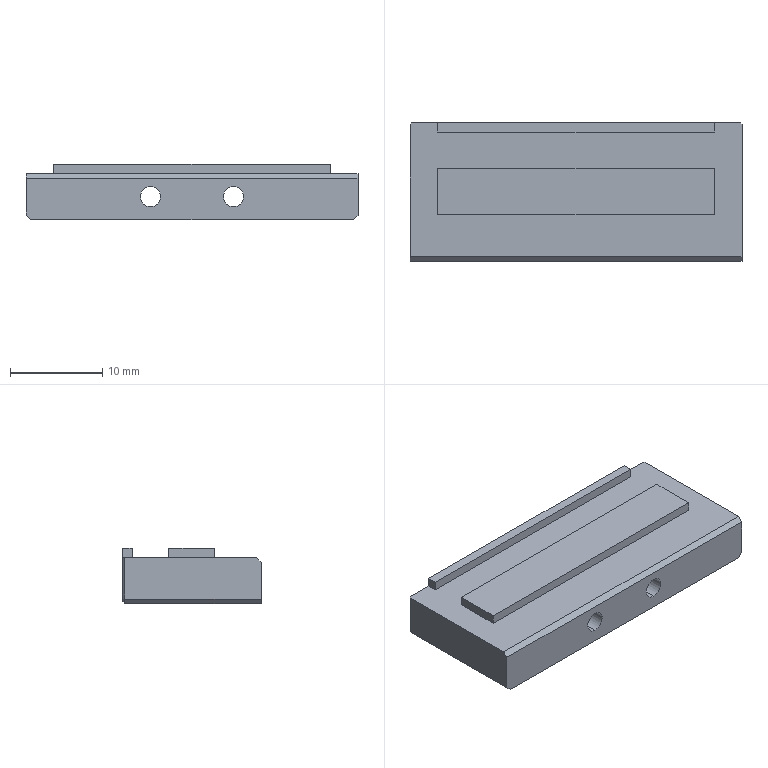Part | SolidWorks | features BaseBody 1 | 1 solid | 49 faces | box 36 x 15 x 6 mm | volume 2606 mm3 | plane 25 | cone 12 | cylinder 12 | commonest cylinder face diameters 2.2 x4 2.5 x4 4 x4
STEP:
#1=CARTESIAN_POINT('',(4.5,14.3,-1.5));
#2=VERTEX_POINT('',#1);
#3=CARTESIAN_POINT('',(4.5,14.3,-5.5));
#4=VERTEX_POINT('',#3);
#5=CARTESIAN_POINT('',(4.5,14.3,-3.5));
#6=DIRECTION('',(0.,-1.,0.));
#7=DIRECTION('',(0.,0.,1.));
#8=AXIS2_PLACEMENT_3D('',#5,#6,#7);
#9=CIRCLE('',#8,2.);
#10=EDGE_CURVE('',#2,#4,#9,.T.);
#11=ORIENTED_EDGE('',*,*,#10,.T.);
#12=CARTESIAN_POINT('',(4.5,14.5,-5.7));
#13=VERTEX_POINT('',#12);
#14=CARTESIAN_POINT('',(4.5,14.3,-5.5));
#15=DIRECTION('',(0.,0.7071,-0.7071));
#16=VECTOR('',#15,1000.);
#17=LINE('',#14,#16);
#18=EDGE_CURVE('',#4,#13,#17,.T.);
#19=ORIENTED_EDGE('',*,*,#18,.T.);
#20=CARTESIAN_POINT('',(4.5,14.5,-1.3));
#21=VERTEX_POINT('',#20);
#22=CARTESIAN_POINT('',(4.5,14.5,-3.5));
#23=DIRECTION('',(0.,1.,0.));
#24=DIRECTION('',(0.,0.,1.));
#25=AXIS2_PLACEMENT_3D('',#22,#23,#24);
#26=CIRCLE('',#25,2.2);
#27=EDGE_CURVE('',#13,#21,#26,.T.);
#28=ORIENTED_EDGE('',*,*,#27,.T.);
#29=CARTESIAN_POINT('',(4.5,14.3,-1.5));
#30=DIRECTION('',(0.,0.7071,0.7071));
#31=VECTOR('',#30,1000.);
#32=LINE('',#29,#31);
#33=EDGE_CURVE('',#2,#21,#32,.T.);
#34=ORIENTED_EDGE('',*,*,#33,.F.);
#35=EDGE_LOOP('',(#11,#19,#28,#34));
#36=FACE_OUTER_BOUND('',#35,.T.);
#37=CARTESIAN_POINT('',(4.5,14.3,-3.5));
#38=DIRECTION('',(0.,1.,0.));
#39=DIRECTION('',(0.,0.,1.));
#40=AXIS2_PLACEMENT_3D('',#37,#38,#39);
#41=CONICAL_SURFACE('',#40,2.,0.7854);
#42=ADVANCED_FACE('',(#36),#41,.F.);
#43=CARTESIAN_POINT('',(4.5,8.5,-1.5));
#44=VERTEX_POINT('',#43);
#45=CARTESIAN_POINT('',(4.5,8.5,-5.5));
#46=VERTEX_POINT('',#45);
#47=CARTESIAN_POINT('',(4.5,8.5,-3.5));
#48=DIRECTION('',(0.,-1.,0.));
#49=DIRECTION('',(0.,0.,1.));
#50=AXIS2_PLACEMENT_3D('',#47,#48,#49);
#51=CIRCLE('',#50,2.);
#52=EDGE_CURVE('',#44,#46,#51,.T.);
#53=ORIENTED_EDGE('',*,*,#52,.T.);
#54=CARTESIAN_POINT('',(4.5,8.5,-5.5));
#55=DIRECTION('',(0.,1.,0.));
#56=VECTOR('',#55,1000.);
#57=LINE('',#54,#56);
#58=EDGE_CURVE('',#46,#4,#57,.T.);
#59=ORIENTED_EDGE('',*,*,#58,.T.);
#60=ORIENTED_EDGE('',*,*,#10,.F.);
#61=CARTESIAN_POINT('',(4.5,8.5,-1.5));
#62=DIRECTION('',(0.,1.,0.));
#63=VECTOR('',#62,1000.);
#64=LINE('',#61,#63);
#65=EDGE_CURVE('',#44,#2,#64,.T.);
#66=ORIENTED_EDGE('',*,*,#65,.F.);
#67=EDGE_LOOP('',(#53,#59,#60,#66));
#68=FACE_OUTER_BOUND('',#67,.T.);
#69=CARTESIAN_POINT('',(4.5,8.5,-3.5));
#70=DIRECTION('',(0.,1.,0.));
#71=DIRECTION('',(0.,0.,1.));
#72=AXIS2_PLACEMENT_3D('',#69,#70,#71);
#73=CYLINDRICAL_SURFACE('',#72,2.);
#74=ADVANCED_FACE('',(#68),#73,.F.);
#75=CARTESIAN_POINT('',(-4.5,14.3,-1.5));
#76=VERTEX_POINT('',#75);
#77=CARTESIAN_POINT('',(-4.5,14.3,-5.5));
#78=VERTEX_POINT('',#77);
#79=CARTESIAN_POINT('',(-4.5,14.3,-3.5));
#80=DIRECTION('',(0.,-1.,0.));
#81=DIRECTION('',(0.,0.,1.));
#82=AXIS2_PLACEMENT_3D('',#79,#80,#81);
#83=CIRCLE('',#82,2.);
#84=EDGE_CURVE('',#76,#78,#83,.T.);
#85=ORIENTED_EDGE('',*,*,#84,.T.);
#86=CARTESIAN_POINT('',(-4.5,14.5,-5.7));
#87=VERTEX_POINT('',#86);
#88=CARTESIAN_POINT('',(-4.5,14.3,-5.5));
#89=DIRECTION('',(0.,0.7071,-0.7071));
#90=VECTOR('',#89,1000.);
#91=LINE('',#88,#90);
#92=EDGE_CURVE('',#78,#87,#91,.T.);
#93=ORIENTED_EDGE('',*,*,#92,.T.);
#94=CARTESIAN_POINT('',(-4.5,14.5,-1.3));
#95=VERTEX_POINT('',#94);
#96=CARTESIAN_POINT('',(-4.5,14.5,-3.5));
#97=DIRECTION('',(0.,-1.,0.));
#98=DIRECTION('',(0.,0.,1.));
#99=AXIS2_PLACEMENT_3D('',#96,#97,#98);
#100=CIRCLE('',#99,2.2);
#101=EDGE_CURVE('',#95,#87,#100,.T.);
#102=ORIENTED_EDGE('',*,*,#101,.F.);
#103=CARTESIAN_POINT('',(-4.5,14.3,-1.5));
#104=DIRECTION('',(0.,0.7071,0.7071));
#105=VECTOR('',#104,1000.);
#106=LINE('',#103,#105);
#107=EDGE_CURVE('',#76,#95,#106,.T.);
#108=ORIENTED_EDGE('',*,*,#107,.F.);
#109=EDGE_LOOP('',(#85,#93,#102,#108));
#110=FACE_OUTER_BOUND('',#109,.T.);
#111=CARTESIAN_POINT('',(-4.5,14.3,-3.5));
#112=DIRECTION('',(0.,1.,0.));
#113=DIRECTION('',(0.,0.,1.));
#114=AXIS2_PLACEMENT_3D('',#111,#112,#113);
#115=CONICAL_SURFACE('',#114,2.,0.7854);
#116=ADVANCED_FACE('',(#110),#115,.F.);
#117=CARTESIAN_POINT('',(-4.5,8.5,-1.5));
#118=VERTEX_POINT('',#117);
#119=CARTESIAN_POINT('',(-4.5,8.5,-5.5));
#120=VERTEX_POINT('',#119);
#121=CARTESIAN_POINT('',(-4.5,8.5,-3.5));
#122=DIRECTION('',(0.,-1.,0.));
#123=DIRECTION('',(0.,0.,1.));
#124=AXIS2_PLACEMENT_3D('',#121,#122,#123);
#125=CIRCLE('',#124,2.);
#126=EDGE_CURVE('',#118,#120,#125,.T.);
#127=ORIENTED_EDGE('',*,*,#126,.T.);
#128=CARTESIAN_POINT('',(-4.5,8.5,-5.5));
#129=DIRECTION('',(0.,1.,0.));
#130=VECTOR('',#129,1000.);
#131=LINE('',#128,#130);
#132=EDGE_CURVE('',#120,#78,#131,.T.);
#133=ORIENTED_EDGE('',*,*,#132,.T.);
#134=ORIENTED_EDGE('',*,*,#84,.F.);
#135=CARTESIAN_POINT('',(-4.5,8.5,-1.5));
#136=DIRECTION('',(0.,1.,0.));
#137=VECTOR('',#136,1000.);
#138=LINE('',#135,#137);
#139=EDGE_CURVE('',#118,#76,#138,.T.);
#140=ORIENTED_EDGE('',*,*,#139,.F.);
#141=EDGE_LOOP('',(#127,#133,#134,#140));
#142=FACE_OUTER_BOUND('',#141,.T.);
#143=CARTESIAN_POINT('',(-4.5,8.5,-3.5));
#144=DIRECTION('',(0.,1.,0.));
#145=DIRECTION('',(0.,0.,1.));
#146=AXIS2_PLACEMENT_3D('',#143,#144,#145);
#147=CYLINDRICAL_SURFACE('',#146,2.);
#148=ADVANCED_FACE('',(#142),#147,.F.);
#149=CARTESIAN_POINT('',(4.5,-0.5,-2.4));
#150=VERTEX_POINT('',#149);
#151=CARTESIAN_POINT('',(4.5,-0.5,-4.6));
#152=VERTEX_POINT('',#151);
#153=CARTESIAN_POINT('',(4.5,-0.5,-3.5));
#154=DIRECTION('',(0.,-1.,0.));
#155=DIRECTION('',(0.,0.,1.));
#156=AXIS2_PLACEMENT_3D('',#153,#154,#155);
#157=CIRCLE('',#156,1.1);
#158=EDGE_CURVE('',#150,#152,#157,.T.);
#159=ORIENTED_EDGE('',*,*,#158,.T.);
#160=CARTESIAN_POINT('',(4.5,8.5,-4.6));
#161=VERTEX_POINT('',#160);
#162=CARTESIAN_POINT('',(4.5,-0.5,-4.6));
#163=DIRECTION('',(0.,1.,0.));
#164=VECTOR('',#163,1000.);
#165=LINE('',#162,#164);
#166=EDGE_CURVE('',#152,#161,#165,.T.);
#167=ORIENTED_EDGE('',*,*,#166,.T.);
#168=CARTESIAN_POINT('',(4.5,8.5,-2.4));
#169=VERTEX_POINT('',#168);
#170=CARTESIAN_POINT('',(4.5,8.5,-3.5));
#171=DIRECTION('',(0.,1.,0.));
#172=DIRECTION('',(0.,0.,1.));
#173=AXIS2_PLACEMENT_3D('',#170,#171,#172);
#174=CIRCLE('',#173,1.1);
#175=EDGE_CURVE('',#161,#169,#174,.T.);
#176=ORIENTED_EDGE('',*,*,#175,.T.);
#177=CARTESIAN_POINT('',(4.5,-0.5,-2.4));
#178=DIRECTION('',(0.,1.,0.));
#179=VECTOR('',#178,1000.);
#180=LINE('',#177,#179);
#181=EDGE_CURVE('',#150,#169,#180,.T.);
#182=ORIENTED_EDGE('',*,*,#181,.F.);
#183=EDGE_LOOP('',(#159,#167,#176,#182));
#184=FACE_OUTER_BOUND('',#183,.T.);
#185=CARTESIAN_POINT('',(4.5,-0.5,-3.5));
#186=DIRECTION('',(0.,1.,0.));
#187=DIRECTION('',(0.,0.,1.));
#188=AXIS2_PLACEMENT_3D('',#185,#186,#187);
#189=CYLINDRICAL_SURFACE('',#188,1.1);
#190=ADVANCED_FACE('',(#184),#189,.F.);
#191=CARTESIAN_POINT('',(-1.25,2.9,-5.75));
#192=VERTEX_POINT('',#191);
#193=CARTESIAN_POINT('',(1.25,2.9,-5.75));
#194=VERTEX_POINT('',#193);
#195=CARTESIAN_POINT('',(0.,2.9,-5.75));
#196=DIRECTION('',(0.,0.,1.));
#197=DIRECTION('',(-1.,0.,0.));
#198=AXIS2_PLACEMENT_3D('',#195,#196,#197);
#199=CIRCLE('',#198,1.25);
#200=EDGE_CURVE('',#192,#194,#199,.T.);
#201=ORIENTED_EDGE('',*,*,#200,.T.);
#202=CARTESIAN_POINT('',(1.5,2.9,-6.));
#203=VERTEX_POINT('',#202);
#204=CARTESIAN_POINT('',(1.25,2.9,-5.75));
#205=DIRECTION('',(0.7071,0.,-0.7071));
#206=VECTOR('',#205,1000.);
#207=LINE('',#204,#206);
#208=EDGE_CURVE('',#194,#203,#207,.T.);
#209=ORIENTED_EDGE('',*,*,#208,.T.);
#210=CARTESIAN_POINT('',(-1.5,2.9,-6.));
#211=VERTEX_POINT('',#210);
#212=CARTESIAN_POINT('',(0.,2.9,-6.));
#213=DIRECTION('',(0.,0.,-1.));
#214=DIRECTION('',(-1.,0.,0.));
#215=AXIS2_PLACEMENT_3D('',#212,#213,#214);
#216=CIRCLE('',#215,1.5);
#217=EDGE_CURVE('',#203,#211,#216,.T.);
#218=ORIENTED_EDGE('',*,*,#217,.T.);
#219=CARTESIAN_POINT('',(-1.25,2.9,-5.75));
#220=DIRECTION('',(-0.7071,0.,-0.7071));
#221=VECTOR('',#220,1000.);
#222=LINE('',#219,#221);
#223=EDGE_CURVE('',#192,#211,#222,.T.);
#224=ORIENTED_EDGE('',*,*,#223,.F.);
#225=EDGE_LOOP('',(#201,#209,#218,#224));
#226=FACE_OUTER_BOUND('',#225,.T.);
#227=CARTESIAN_POINT('',(0.,2.9,-5.75));
#228=DIRECTION('',(0.,0.,-1.));
#229=DIRECTION('',(-1.,0.,0.));
#230=AXIS2_PLACEMENT_3D('',#227,#228,#229);
#231=CONICAL_SURFACE('',#230,1.25,0.7854);
#232=ADVANCED_FACE('',(#226),#231,.F.);
#233=CARTESIAN_POINT('',(-1.25,11.9,-5.75));
#234=VERTEX_POINT('',#233);
#235=CARTESIAN_POINT('',(1.25,11.9,-5.75));
#236=VERTEX_POINT('',#235);
#237=CARTESIAN_POINT('',(0.,11.9,-5.75));
#238=DIRECTION('',(0.,0.,1.));
#239=DIRECTION('',(-1.,0.,0.));
#240=AXIS2_PLACEMENT_3D('',#237,#238,#239);
#241=CIRCLE('',#240,1.25);
#242=EDGE_CURVE('',#234,#236,#241,.T.);
#243=ORIENTED_EDGE('',*,*,#242,.T.);
#244=CARTESIAN_POINT('',(1.5,11.9,-6.));
#245=VERTEX_POINT('',#244);
#246=CARTESIAN_POINT('',(1.25,11.9,-5.75));
#247=DIRECTION('',(0.7071,0.,-0.7071));
#248=VECTOR('',#247,1000.);
#249=LINE('',#246,#248);
#250=EDGE_CURVE('',#236,#245,#249,.T.);
#251=ORIENTED_EDGE('',*,*,#250,.T.);
#252=CARTESIAN_POINT('',(-1.5,11.9,-6.));
#253=VERTEX_POINT('',#252);
#254=CARTESIAN_POINT('',(0.,11.9,-6.));
#255=DIRECTION('',(0.,0.,-1.));
#256=DIRECTION('',(-1.,0.,0.));
#257=AXIS2_PLACEMENT_3D('',#254,#255,#256);
#258=CIRCLE('',#257,1.5);
#259=EDGE_CURVE('',#245,#253,#258,.T.);
#260=ORIENTED_EDGE('',*,*,#259,.T.);
#261=CARTESIAN_POINT('',(-1.25,11.9,-5.75));
#262=DIRECTION('',(-0.7071,0.,-0.7071));
#263=VECTOR('',#262,1000.);
#264=LINE('',#261,#263);
#265=EDGE_CURVE('',#234,#253,#264,.T.);
#266=ORIENTED_EDGE('',*,*,#265,.F.);
#267=EDGE_LOOP('',(#243,#251,#260,#266));
#268=FACE_OUTER_BOUND('',#267,.T.);
#269=CARTESIAN_POINT('',(0.,11.9,-5.75));
#270=DIRECTION('',(0.,0.,-1.));
#271=DIRECTION('',(-1.,0.,0.));
#272=AXIS2_PLACEMENT_3D('',#269,#270,#271);
#273=CONICAL_SURFACE('',#272,1.25,0.7854);
#274=ADVANCED_FACE('',(#268),#273,.F.);
#275=CARTESIAN_POINT('',(-4.5,-0.5,-4.6));
#276=VERTEX_POINT('',#275);
#277=CARTESIAN_POINT('',(-4.5,-0.5,-2.4));
#278=VERTEX_POINT('',#277);
#279=CARTESIAN_POINT('',(-4.5,-0.5,-3.5));
#280=DIRECTION('',(0.,1.,0.));
#281=DIRECTION('',(0.,0.,1.));
#282=AXIS2_PLACEMENT_3D('',#279,#280,#281);
#283=CIRCLE('',#282,1.1);
#284=EDGE_CURVE('',#276,#278,#283,.T.);
#285=ORIENTED_EDGE('',*,*,#284,.F.);
#286=CARTESIAN_POINT('',(-4.5,8.5,-4.6));
#287=VERTEX_POINT('',#286);
#288=CARTESIAN_POINT('',(-4.5,-0.5,-4.6));
#289=DIRECTION('',(0.,1.,0.));
#290=VECTOR('',#289,1000.);
#291=LINE('',#288,#290);
#292=EDGE_CURVE('',#276,#287,#291,.T.);
#293=ORIENTED_EDGE('',*,*,#292,.T.);
#294=CARTESIAN_POINT('',(-4.5,8.5,-2.4));
#295=VERTEX_POINT('',#294);
#296=CARTESIAN_POINT('',(-4.5,8.5,-3.5));
#297=DIRECTION('',(0.,1.,0.));
#298=DIRECTION('',(0.,0.,1.));
#299=AXIS2_PLACEMENT_3D('',#296,#297,#298);
#300=CIRCLE('',#299,1.1);
#301=EDGE_CURVE('',#287,#295,#300,.T.);
#302=ORIENTED_EDGE('',*,*,#301,.T.);
#303=CARTESIAN_POINT('',(-4.5,-0.5,-2.4));
#304=DIRECTION('',(0.,1.,0.));
#305=VECTOR('',#304,1000.);
#306=LINE('',#303,#305);
#307=EDGE_CURVE('',#278,#295,#306,.T.);
#308=ORIENTED_EDGE('',*,*,#307,.F.);
#309=EDGE_LOOP('',(#285,#293,#302,#308));
#310=FACE_OUTER_BOUND('',#309,.T.);
#311=CARTESIAN_POINT('',(-4.5,-0.5,-3.5));
#312=DIRECTION('',(0.,1.,0.));
#313=DIRECTION('',(0.,0.,1.));
#314=AXIS2_PLACEMENT_3D('',#311,#312,#313);
#315=CYLINDRICAL_SURFACE('',#314,1.1);
#316=ADVANCED_FACE('',(#310),#315,.F.);
#317=CARTESIAN_POINT('',(-1.25,2.9,-2.));
#318=VERTEX_POINT('',#317);
#319=CARTESIAN_POINT('',(1.25,2.9,-2.));
#320=VERTEX_POINT('',#319);
#321=CARTESIAN_POINT('',(0.,2.9,-2.));
#322=DIRECTION('',(0.,0.,1.));
#323=DIRECTION('',(-1.,0.,0.));
#324=AXIS2_PLACEMENT_3D('',#321,#322,#323);
#325=CIRCLE('',#324,1.25);
#326=EDGE_CURVE('',#318,#320,#325,.T.);
#327=ORIENTED_EDGE('',*,*,#326,.T.);
#328=CARTESIAN_POINT('',(1.25,2.9,-2.));
#329=DIRECTION('',(0.,0.,-1.));
#330=VECTOR('',#329,1000.);
#331=LINE('',#328,#330);
#332=EDGE_CURVE('',#320,#194,#331,.T.);
#333=ORIENTED_EDGE('',*,*,#332,.T.);
#334=ORIENTED_EDGE('',*,*,#200,.F.);
#335=CARTESIAN_POINT('',(-1.25,2.9,-2.));
#336=DIRECTION('',(0.,0.,-1.));
#337=VECTOR('',#336,1000.);
#338=LINE('',#335,#337);
#339=EDGE_CURVE('',#318,#192,#338,.T.);
#340=ORIENTED_EDGE('',*,*,#339,.F.);
#341=EDGE_LOOP('',(#327,#333,#334,#340));
#342=FACE_OUTER_BOUND('',#341,.T.);
#343=CARTESIAN_POINT('',(0.,2.9,-2.));
#344=DIRECTION('',(0.,0.,-1.));
#345=DIRECTION('',(-1.,0.,0.));
#346=AXIS2_PLACEMENT_3D('',#343,#344,#345);
#347=CYLINDRICAL_SURFACE('',#346,1.25);
#348=ADVANCED_FACE('',(#342),#347,.F.);
#349=CARTESIAN_POINT('',(-1.25,11.9,-2.));
#350=VERTEX_POINT('',#349);
#351=CARTESIAN_POINT('',(1.25,11.9,-2.));
#352=VERTEX_POINT('',#351);
#353=CARTESIAN_POINT('',(0.,11.9,-2.));
#354=DIRECTION('',(0.,0.,1.));
#355=DIRECTION('',(-1.,0.,0.));
#356=AXIS2_PLACEMENT_3D('',#353,#354,#355);
#357=CIRCLE('',#356,1.25);
#358=EDGE_CURVE('',#350,#352,#357,.T.);
#359=ORIENTED_EDGE('',*,*,#358,.T.);
#360=CARTESIAN_POINT('',(1.25,11.9,-2.));
#361=DIRECTION('',(0.,0.,-1.));
#362=VECTOR('',#361,1000.);
#363=LINE('',#360,#362);
#364=EDGE_CURVE('',#352,#236,#363,.T.);
#365=ORIENTED_EDGE('',*,*,#364,.T.);
#366=ORIENTED_EDGE('',*,*,#242,.F.);
#367=CARTESIAN_POINT('',(-1.25,11.9,-2.));
#368=DIRECTION('',(0.,0.,-1.));
#369=VECTOR('',#368,1000.);
#370=LINE('',#367,#369);
#371=EDGE_CURVE('',#350,#234,#370,.T.);
#372=ORIENTED_EDGE('',*,*,#371,.F.);
#373=EDGE_LOOP('',(#359,#365,#366,#372));
#374=FACE_OUTER_BOUND('',#373,.T.);
#375=CARTESIAN_POINT('',(0.,11.9,-2.));
#376=DIRECTION('',(0.,0.,-1.));
#377=DIRECTION('',(-1.,0.,0.));
#378=AXIS2_PLACEMENT_3D('',#375,#376,#377);
#379=CYLINDRICAL_SURFACE('',#378,1.25);
#380=ADVANCED_FACE('',(#374),#379,.F.);
#381=CARTESIAN_POINT('',(0.,2.9,-1.249));
#382=VERTEX_POINT('',#381);
#383=CARTESIAN_POINT('',(0.,2.9,-1.249));
#384=DIRECTION('',(-0.8572,0.,-0.515));
#385=VECTOR('',#384,1000.);
#386=LINE('',#383,#385);
#387=EDGE_CURVE('',#382,#318,#386,.T.);
#388=ORIENTED_EDGE('',*,*,#387,.F.);
#389=CARTESIAN_POINT('',(0.,2.9,-1.249));
#390=DIRECTION('',(0.8572,0.,-0.515));
#391=VECTOR('',#390,1000.);
#392=LINE('',#389,#391);
#393=EDGE_CURVE('',#382,#320,#392,.T.);
#394=ORIENTED_EDGE('',*,*,#393,.T.);
#395=ORIENTED_EDGE('',*,*,#326,.F.);
#396=EDGE_LOOP('',(#388,#394,#395));
#397=FACE_OUTER_BOUND('',#396,.T.);
#398=CARTESIAN_POINT('',(0.,2.9,-1001.249));
#399=DIRECTION('',(0.,0.,-1.));
#400=DIRECTION('',(-1.,0.,0.));
#401=AXIS2_PLACEMENT_3D('',#398,#399,#400);
#402=CONICAL_SURFACE('',#401,1664.279,1.03);
#403=ADVANCED_FACE('',(#397),#402,.F.);
#404=CARTESIAN_POINT('',(0.,11.9,-1.249));
#405=VERTEX_POINT('',#404);
#406=CARTESIAN_POINT('',(0.,11.9,-1.249));
#407=DIRECTION('',(-0.8572,0.,-0.515));
#408=VECTOR('',#407,1000.);
#409=LINE('',#406,#408);
#410=EDGE_CURVE('',#405,#350,#409,.T.);
#411=ORIENTED_EDGE('',*,*,#410,.F.);
#412=CARTESIAN_POINT('',(0.,11.9,-1.249));
#413=DIRECTION('',(0.8572,0.,-0.515));
#414=VECTOR('',#413,1000.);
#415=LINE('',#412,#414);
#416=EDGE_CURVE('',#405,#352,#415,.T.);
#417=ORIENTED_EDGE('',*,*,#416,.T.);
#418=ORIENTED_EDGE('',*,*,#358,.F.);
#419=EDGE_LOOP('',(#411,#417,#418));
#420=FACE_OUTER_BOUND('',#419,.T.);
#421=CARTESIAN_POINT('',(0.,11.9,-1001.249));
#422=DIRECTION('',(0.,0.,-1.));
#423=DIRECTION('',(-1.,0.,0.));
#424=AXIS2_PLACEMENT_3D('',#421,#422,#423);
#425=CONICAL_SURFACE('',#424,1664.279,1.03);
#426=ADVANCED_FACE('',(#420),#425,.F.);
#427=ORIENTED_EDGE('',*,*,#18,.F.);
#428=CARTESIAN_POINT('',(4.5,14.3,-3.5));
#429=DIRECTION('',(0.,-1.,0.));
#430=DIRECTION('',(0.,0.,1.));
#431=AXIS2_PLACEMENT_3D('',#428,#429,#430);
#432=CIRCLE('',#431,2.);
#433=EDGE_CURVE('',#4,#2,#432,.T.);
#434=ORIENTED_EDGE('',*,*,#433,.T.);
#435=ORIENTED_EDGE('',*,*,#33,.T.);
#436=CARTESIAN_POINT('',(4.5,14.5,-3.5));
#437=DIRECTION('',(0.,1.,0.));
#438=DIRECTION('',(0.,0.,1.));
#439=AXIS2_PLACEMENT_3D('',#436,#437,#438);
#440=CIRCLE('',#439,2.2);
#441=EDGE_CURVE('',#21,#13,#440,.T.);
#442=ORIENTED_EDGE('',*,*,#441,.T.);
#443=EDGE_LOOP('',(#427,#434,#435,#442));
#444=FACE_OUTER_BOUND('',#443,.T.);
#445=CARTESIAN_POINT('',(4.5,14.3,-3.5));
#446=DIRECTION('',(0.,1.,0.));
#447=DIRECTION('',(0.,0.,1.));
#448=AXIS2_PLACEMENT_3D('',#445,#446,#447);
#449=CONICAL_SURFACE('',#448,2.,0.7854);
#450=ADVANCED_FACE('',(#444),#449,.F.);
#451=ORIENTED_EDGE('',*,*,#101,.T.);
#452=CARTESIAN_POINT('',(-4.5,14.5,-3.5));
#453=DIRECTION('',(0.,-1.,0.));
#454=DIRECTION('',(0.,0.,1.));
#455=AXIS2_PLACEMENT_3D('',#452,#453,#454);
#456=CIRCLE('',#455,2.2);
#457=EDGE_CURVE('',#87,#95,#456,.T.);
#458=ORIENTED_EDGE('',*,*,#457,.T.);
#459=EDGE_LOOP('',(#451,#458));
#460=FACE_BOUND('',#459,.T.);
#461=ORIENTED_EDGE('',*,*,#441,.F.);
#462=ORIENTED_EDGE('',*,*,#27,.F.);
#463=EDGE_LOOP('',(#461,#462));
#464=FACE_BOUND('',#463,.T.);
#465=CARTESIAN_POINT('',(17.8,14.5,-5.417));
#466=VERTEX_POINT('',#465);
#467=CARTESIAN_POINT('',(17.417,14.5,-5.8));
#468=VERTEX_POINT('',#467);
#469=CARTESIAN_POINT('',(17.8,14.5,-5.417));
#470=DIRECTION('',(-0.7071,0.,-0.7071));
#471=VECTOR('',#470,1000.);
#472=LINE('',#469,#471);
#473=EDGE_CURVE('',#466,#468,#472,.T.);
#474=ORIENTED_EDGE('',*,*,#473,.T.);
#475=CARTESIAN_POINT('',(-17.417,14.5,-5.8));
#476=VERTEX_POINT('',#475);
#477=CARTESIAN_POINT('',(0.,14.5,-5.8));
#478=DIRECTION('',(-1.,0.,0.));
#479=VECTOR('',#478,1000.);
#480=LINE('',#477,#479);
#481=EDGE_CURVE('',#468,#476,#480,.T.);
#482=ORIENTED_EDGE('',*,*,#481,.T.);
#483=CARTESIAN_POINT('',(-17.8,14.5,-5.417));
#484=VERTEX_POINT('',#483);
#485=CARTESIAN_POINT('',(-17.417,14.5,-5.8));
#486=DIRECTION('',(-0.7071,0.,0.7071));
#487=VECTOR('',#486,1000.);
#488=LINE('',#485,#487);
#489=EDGE_CURVE('',#476,#484,#488,.T.);
#490=ORIENTED_EDGE('',*,*,#489,.T.);
#491=CARTESIAN_POINT('',(-17.8,14.5,-1.));
#492=VERTEX_POINT('',#491);
#493=CARTESIAN_POINT('',(-17.8,14.5,-2.9));
#494=DIRECTION('',(0.,0.,1.));
#495=VECTOR('',#494,1000.);
#496=LINE('',#493,#495);
#497=EDGE_CURVE('',#484,#492,#496,.T.);
#498=ORIENTED_EDGE('',*,*,#497,.T.);
#499=CARTESIAN_POINT('',(-15.,14.5,-1.));
#500=VERTEX_POINT('',#499);
#501=CARTESIAN_POINT('',(0.,14.5,-1.));
#502=DIRECTION('',(1.,0.,0.));
#503=VECTOR('',#502,1000.);
#504=LINE('',#501,#503);
#505=EDGE_CURVE('',#492,#500,#504,.T.);
#506=ORIENTED_EDGE('',*,*,#505,.T.);
#507=CARTESIAN_POINT('',(-15.,14.5,0.));
#508=VERTEX_POINT('',#507);
#509=CARTESIAN_POINT('',(-15.,14.5,-2.9));
#510=DIRECTION('',(0.,0.,1.));
#511=VECTOR('',#510,1000.);
#512=LINE('',#509,#511);
#513=EDGE_CURVE('',#500,#508,#512,.T.);
#514=ORIENTED_EDGE('',*,*,#513,.T.);
#515=CARTESIAN_POINT('',(15.,14.5,0.));
#516=VERTEX_POINT('',#515);
#517=CARTESIAN_POINT('',(0.,14.5,0.));
#518=DIRECTION('',(1.,0.,0.));
#519=VECTOR('',#518,1000.);
#520=LINE('',#517,#519);
#521=EDGE_CURVE('',#508,#516,#520,.T.);
#522=ORIENTED_EDGE('',*,*,#521,.T.);
#523=CARTESIAN_POINT('',(15.,14.5,-1.));
#524=VERTEX_POINT('',#523);
#525=CARTESIAN_POINT('',(15.,14.5,-2.9));
#526=DIRECTION('',(0.,0.,-1.));
#527=VECTOR('',#526,1000.);
#528=LINE('',#525,#527);
#529=EDGE_CURVE('',#516,#524,#528,.T.);
#530=ORIENTED_EDGE('',*,*,#529,.T.);
#531=CARTESIAN_POINT('',(17.8,14.5,-1.));
#532=VERTEX_POINT('',#531);
#533=CARTESIAN_POINT('',(0.,14.5,-1.));
#534=DIRECTION('',(1.,0.,0.));
#535=VECTOR('',#534,1000.);
#536=LINE('',#533,#535);
#537=EDGE_CURVE('',#524,#532,#536,.T.);
#538=ORIENTED_EDGE('',*,*,#537,.T.);
#539=CARTESIAN_POINT('',(17.8,14.5,-2.9));
#540=DIRECTION('',(0.,0.,-1.));
#541=VECTOR('',#540,1000.);
#542=LINE('',#539,#541);
#543=EDGE_CURVE('',#532,#466,#542,.T.);
#544=ORIENTED_EDGE('',*,*,#543,.T.);
#545=EDGE_LOOP('',(#474,#482,#490,#498,#506,#514,#522,#530,#538,#544));
#546=FACE_OUTER_BOUND('',#545,.T.);
#547=CARTESIAN_POINT('',(-17.8,14.5,-5.8));
#548=DIRECTION('',(0.,1.,0.));
#549=DIRECTION('',(0.,0.,1.));
#550=AXIS2_PLACEMENT_3D('',#547,#548,#549);
#551=PLANE('',#550);
#552=ADVANCED_FACE('',(#460,#464,#546),#551,.T.);
#553=ORIENTED_EDGE('',*,*,#58,.F.);
#554=CARTESIAN_POINT('',(4.5,8.5,-3.5));
#555=DIRECTION('',(0.,-1.,0.));
#556=DIRECTION('',(0.,0.,1.));
#557=AXIS2_PLACEMENT_3D('',#554,#555,#556);
#558=CIRCLE('',#557,2.);
#559=EDGE_CURVE('',#46,#44,#558,.T.);
#560=ORIENTED_EDGE('',*,*,#559,.T.);
#561=ORIENTED_EDGE('',*,*,#65,.T.);
#562=ORIENTED_EDGE('',*,*,#433,.F.);
#563=EDGE_LOOP('',(#553,#560,#561,#562));
#564=FACE_OUTER_BOUND('',#563,.T.);
#565=CARTESIAN_POINT('',(4.5,8.5,-3.5));
#566=DIRECTION('',(0.,1.,0.));
#567=DIRECTION('',(0.,0.,1.));
#568=AXIS2_PLACEMENT_3D('',#565,#566,#567);
#569=CYLINDRICAL_SURFACE('',#568,2.);
#570=ADVANCED_FACE('',(#564),#569,.F.);
#571=ORIENTED_EDGE('',*,*,#92,.F.);
#572=CARTESIAN_POINT('',(-4.5,14.3,-3.5));
#573=DIRECTION('',(0.,-1.,0.));
#574=DIRECTION('',(0.,0.,1.));
#575=AXIS2_PLACEMENT_3D('',#572,#573,#574);
#576=CIRCLE('',#575,2.);
#577=EDGE_CURVE('',#78,#76,#576,.T.);
#578=ORIENTED_EDGE('',*,*,#577,.T.);
#579=ORIENTED_EDGE('',*,*,#107,.T.);
#580=ORIENTED_EDGE('',*,*,#457,.F.);
#581=EDGE_LOOP('',(#571,#578,#579,#580));
#582=FACE_OUTER_BOUND('',#581,.T.);
#583=CARTESIAN_POINT('',(-4.5,14.3,-3.5));
#584=DIRECTION('',(0.,1.,0.));
#585=DIRECTION('',(0.,0.,1.));
#586=AXIS2_PLACEMENT_3D('',#583,#584,#585);
#587=CONICAL_SURFACE('',#586,2.,0.7854);
#588=ADVANCED_FACE('',(#582),#587,.F.);
#589=CARTESIAN_POINT('',(-17.5,14.3,-6.));
#590=VERTEX_POINT('',#589);
#591=CARTESIAN_POINT('',(-17.5,14.3,-6.));
#592=DIRECTION('',(0.2811,0.6786,0.6786));
#593=VECTOR('',#592,1000.);
#594=LINE('',#591,#593);
#595=EDGE_CURVE('',#590,#476,#594,.T.);
#596=ORIENTED_EDGE('',*,*,#595,.T.);
#597=ORIENTED_EDGE('',*,*,#481,.F.);
#598=CARTESIAN_POINT('',(17.5,14.3,-6.));
#599=VERTEX_POINT('',#598);
#600=CARTESIAN_POINT('',(17.417,14.5,-5.8));
#601=DIRECTION('',(0.2811,-0.6786,-0.6786));
#602=VECTOR('',#601,1000.);
#603=LINE('',#600,#602);
#604=EDGE_CURVE('',#468,#599,#603,.T.);
#605=ORIENTED_EDGE('',*,*,#604,.T.);
#606=CARTESIAN_POINT('',(0.,14.3,-6.));
#607=DIRECTION('',(-1.,0.,0.));
#608=VECTOR('',#607,1000.);
#609=LINE('',#606,#608);
#610=EDGE_CURVE('',#599,#590,#609,.T.);
#611=ORIENTED_EDGE('',*,*,#610,.T.);
#612=EDGE_LOOP('',(#596,#597,#605,#611));
#613=FACE_OUTER_BOUND('',#612,.T.);
#614=CARTESIAN_POINT('',(-17.71,14.5,-5.8));
#615=DIRECTION('',(0.,0.7071,-0.7071));
#616=DIRECTION('',(1.,0.,0.));
#617=AXIS2_PLACEMENT_3D('',#614,#615,#616);
#618=PLANE('',#617);
#619=ADVANCED_FACE('',(#613),#618,.T.);
#620=CARTESIAN_POINT('',(18.,14.3,-5.5));
#621=VERTEX_POINT('',#620);
#622=CARTESIAN_POINT('',(17.75,14.3,-5.75));
#623=DIRECTION('',(0.7071,0.,0.7071));
#624=VECTOR('',#623,1000.);
#625=LINE('',#622,#624);
#626=EDGE_CURVE('',#599,#621,#625,.T.);
#627=ORIENTED_EDGE('',*,*,#626,.F.);
#628=ORIENTED_EDGE('',*,*,#604,.F.);
#629=ORIENTED_EDGE('',*,*,#473,.F.);
#630=CARTESIAN_POINT('',(18.,14.3,-5.5));
#631=DIRECTION('',(-0.6786,0.6786,0.2811));
#632=VECTOR('',#631,1000.);
#633=LINE('',#630,#632);
#634=EDGE_CURVE('',#621,#466,#633,.T.);
#635=ORIENTED_EDGE('',*,*,#634,.F.);
#636=EDGE_LOOP('',(#627,#628,#629,#635));
#637=FACE_OUTER_BOUND('',#636,.T.);
#638=CARTESIAN_POINT('',(17.862,14.5,-5.356));
#639=DIRECTION('',(-0.5,-0.7071,0.5));
#640=DIRECTION('',(-0.7071,0.,-0.7071));
#641=AXIS2_PLACEMENT_3D('',#638,#639,#640);
#642=PLANE('',#641);
#643=ADVANCED_FACE('',(#637),#642,.F.);
#644=CARTESIAN_POINT('',(18.,14.3,-1.));
#645=VERTEX_POINT('',#644);
#646=CARTESIAN_POINT('',(18.,14.3,-3.264));
#647=DIRECTION('',(0.,0.,1.));
#648=VECTOR('',#647,1000.);
#649=LINE('',#646,#648);
#650=EDGE_CURVE('',#621,#645,#649,.T.);
#651=ORIENTED_EDGE('',*,*,#650,.F.);
#652=ORIENTED_EDGE('',*,*,#634,.T.);
#653=ORIENTED_EDGE('',*,*,#543,.F.);
#654=CARTESIAN_POINT('',(17.9,14.4,-1.));
#655=DIRECTION('',(-0.7071,0.7071,0.));
#656=VECTOR('',#655,1000.);
#657=LINE('',#654,#656);
#658=EDGE_CURVE('',#645,#532,#657,.T.);
#659=ORIENTED_EDGE('',*,*,#658,.F.);
#660=EDGE_LOOP('',(#651,#652,#653,#659));
#661=FACE_OUTER_BOUND('',#660,.T.);
#662=CARTESIAN_POINT('',(18.,14.3,-5.527));
#663=DIRECTION('',(-0.7071,-0.7071,0.));
#664=DIRECTION('',(0.,0.,1.));
#665=AXIS2_PLACEMENT_3D('',#662,#663,#664);
#666=PLANE('',#665);
#667=ADVANCED_FACE('',(#661),#666,.F.);
#668=CARTESIAN_POINT('',(-15.,9.5,-1.));
#669=VERTEX_POINT('',#668);
#670=CARTESIAN_POINT('',(15.,9.5,-1.));
#671=VERTEX_POINT('',#670);
#672=CARTESIAN_POINT('',(0.,9.5,-1.));
#673=DIRECTION('',(1.,0.,0.));
#674=VECTOR('',#673,1000.);
#675=LINE('',#672,#674);
#676=EDGE_CURVE('',#669,#671,#675,.T.);
#677=ORIENTED_EDGE('',*,*,#676,.T.);
#678=CARTESIAN_POINT('',(15.,4.6,-1.));
#679=VERTEX_POINT('',#678);
#680=CARTESIAN_POINT('',(15.,7.25,-1.));
#681=DIRECTION('',(0.,-1.,0.));
#682=VECTOR('',#681,1000.);
#683=LINE('',#680,#682);
#684=EDGE_CURVE('',#671,#679,#683,.T.);
#685=ORIENTED_EDGE('',*,*,#684,.T.);
#686=CARTESIAN_POINT('',(-15.,4.6,-1.));
#687=VERTEX_POINT('',#686);
#688=CARTESIAN_POINT('',(0.,4.6,-1.));
#689=DIRECTION('',(-1.,0.,0.));
#690=VECTOR('',#689,1000.);
#691=LINE('',#688,#690);
#692=EDGE_CURVE('',#679,#687,#691,.T.);
#693=ORIENTED_EDGE('',*,*,#692,.T.);
#694=CARTESIAN_POINT('',(-15.,7.25,-1.));
#695=DIRECTION('',(0.,1.,0.));
#696=VECTOR('',#695,1000.);
#697=LINE('',#694,#696);
#698=EDGE_CURVE('',#687,#669,#697,.T.);
#699=ORIENTED_EDGE('',*,*,#698,.T.);
#700=EDGE_LOOP('',(#677,#685,#693,#699));
#701=FACE_BOUND('',#700,.T.);
#702=CARTESIAN_POINT('',(15.,13.5,-1.));
#703=VERTEX_POINT('',#702);
#704=CARTESIAN_POINT('',(-15.,13.5,-1.));
#705=VERTEX_POINT('',#704);
#706=CARTESIAN_POINT('',(0.,13.5,-1.));
#707=DIRECTION('',(-1.,0.,0.));
#708=VECTOR('',#707,1000.);
#709=LINE('',#706,#708);
#710=EDGE_CURVE('',#703,#705,#709,.T.);
#711=ORIENTED_EDGE('',*,*,#710,.T.);
#712=CARTESIAN_POINT('',(-15.,7.25,-1.));
#713=DIRECTION('',(0.,1.,0.));
#714=VECTOR('',#713,1000.);
#715=LINE('',#712,#714);
#716=EDGE_CURVE('',#705,#500,#715,.T.);
#717=ORIENTED_EDGE('',*,*,#716,.T.);
#718=ORIENTED_EDGE('',*,*,#505,.F.);
#719=CARTESIAN_POINT('',(-18.,14.3,-1.));
#720=VERTEX_POINT('',#719);
#721=CARTESIAN_POINT('',(-17.8,14.5,-1.));
#722=DIRECTION('',(-0.7071,-0.7071,0.));
#723=VECTOR('',#722,1000.);
#724=LINE('',#721,#723);
#725=EDGE_CURVE('',#492,#720,#724,.T.);
#726=ORIENTED_EDGE('',*,*,#725,.T.);
#727=CARTESIAN_POINT('',(-18.,0.000000002,-1.));
#728=VERTEX_POINT('',#727);
#729=CARTESIAN_POINT('',(-18.,7.25,-1.));
#730=DIRECTION('',(0.,-1.,0.));
#731=VECTOR('',#730,1000.);
#732=LINE('',#729,#731);
#733=EDGE_CURVE('',#720,#728,#732,.T.);
#734=ORIENTED_EDGE('',*,*,#733,.T.);
#735=CARTESIAN_POINT('',(18.,0.000000002,-1.));
#736=VERTEX_POINT('',#735);
#737=CARTESIAN_POINT('',(0.,0.,-1.));
#738=DIRECTION('',(1.,0.,0.));
#739=VECTOR('',#738,1000.);
#740=LINE('',#737,#739);
#741=EDGE_CURVE('',#728,#736,#740,.T.);
#742=ORIENTED_EDGE('',*,*,#741,.T.);
#743=CARTESIAN_POINT('',(18.,7.25,-1.));
#744=DIRECTION('',(0.,1.,0.));
#745=VECTOR('',#744,1000.);
#746=LINE('',#743,#745);
#747=EDGE_CURVE('',#736,#645,#746,.T.);
#748=ORIENTED_EDGE('',*,*,#747,.T.);
#749=ORIENTED_EDGE('',*,*,#658,.T.);
#750=ORIENTED_EDGE('',*,*,#537,.F.);
#751=CARTESIAN_POINT('',(15.,7.25,-1.));
#752=DIRECTION('',(0.,-1.,0.));
#753=VECTOR('',#752,1000.);
#754=LINE('',#751,#753);
#755=EDGE_CURVE('',#524,#703,#754,.T.);
#756=ORIENTED_EDGE('',*,*,#755,.T.);
#757=EDGE_LOOP('',(#711,#717,#718,#726,#734,#742,#748,#749,#750,#756));
#758=FACE_OUTER_BOUND('',#757,.T.);
#759=CARTESIAN_POINT('',(-18.,0.,-1.));
#760=DIRECTION('',(0.,0.,1.));
#761=DIRECTION('',(1.,0.,0.));
#762=AXIS2_PLACEMENT_3D('',#759,#760,#761);
#763=PLANE('',#762);
#764=ADVANCED_FACE('',(#701,#758),#763,.T.);
#765=ORIENTED_EDGE('',*,*,#529,.F.);
#766=CARTESIAN_POINT('',(15.,13.5,0.));
#767=VERTEX_POINT('',#766);
#768=CARTESIAN_POINT('',(15.,14.,0.));
#769=DIRECTION('',(0.,1.,0.));
#770=VECTOR('',#769,1000.);
#771=LINE('',#768,#770);
#772=EDGE_CURVE('',#767,#516,#771,.T.);
#773=ORIENTED_EDGE('',*,*,#772,.F.);
#774=CARTESIAN_POINT('',(15.,13.5,-0.5));
#775=DIRECTION('',(0.,0.,1.));
#776=VECTOR('',#775,1000.);
#777=LINE('',#774,#776);
#778=EDGE_CURVE('',#703,#767,#777,.T.);
#779=ORIENTED_EDGE('',*,*,#778,.F.);
#780=ORIENTED_EDGE('',*,*,#755,.F.);
#781=EDGE_LOOP('',(#765,#773,#779,#780));
#782=FACE_OUTER_BOUND('',#781,.T.);
#783=CARTESIAN_POINT('',(15.,13.5,-1.));
#784=DIRECTION('',(-1.,0.,0.));
#785=DIRECTION('',(0.,0.,1.));
#786=AXIS2_PLACEMENT_3D('',#783,#784,#785);
#787=PLANE('',#786);
#788=ADVANCED_FACE('',(#782),#787,.F.);
#789=ORIENTED_EDGE('',*,*,#772,.T.);
#790=ORIENTED_EDGE('',*,*,#521,.F.);
#791=CARTESIAN_POINT('',(-15.,13.5,0.));
#792=VERTEX_POINT('',#791);
#793=CARTESIAN_POINT('',(-15.,14.,0.));
#794=DIRECTION('',(0.,1.,0.));
#795=VECTOR('',#794,1000.);
#796=LINE('',#793,#795);
#797=EDGE_CURVE('',#792,#508,#796,.T.);
#798=ORIENTED_EDGE('',*,*,#797,.F.);
#799=CARTESIAN_POINT('',(0.,13.5,0.));
#800=DIRECTION('',(-1.,0.,0.));
#801=VECTOR('',#800,1000.);
#802=LINE('',#799,#801);
#803=EDGE_CURVE('',#767,#792,#802,.T.);
#804=ORIENTED_EDGE('',*,*,#803,.F.);
#805=EDGE_LOOP('',(#789,#790,#798,#804));
#806=FACE_OUTER_BOUND('',#805,.T.);
#807=CARTESIAN_POINT('',(15.,13.5,0.));
#808=DIRECTION('',(0.,0.,-1.));
#809=DIRECTION('',(-1.,0.,0.));
#810=AXIS2_PLACEMENT_3D('',#807,#808,#809);
#811=PLANE('',#810);
#812=ADVANCED_FACE('',(#806),#811,.F.);
#813=CARTESIAN_POINT('',(-15.,13.5,-0.5));
#814=DIRECTION('',(0.,0.,-1.));
#815=VECTOR('',#814,1000.);
#816=LINE('',#813,#815);
#817=EDGE_CURVE('',#792,#705,#816,.T.);
#818=ORIENTED_EDGE('',*,*,#817,.F.);
#819=ORIENTED_EDGE('',*,*,#797,.T.);
#820=ORIENTED_EDGE('',*,*,#513,.F.);
#821=ORIENTED_EDGE('',*,*,#716,.F.);
#822=EDGE_LOOP('',(#818,#819,#820,#821));
#823=FACE_OUTER_BOUND('',#822,.T.);
#824=CARTESIAN_POINT('',(-15.,13.5,0.));
#825=DIRECTION('',(1.,0.,0.));
#826=DIRECTION('',(0.,0.,-1.));
#827=AXIS2_PLACEMENT_3D('',#824,#825,#826);
#828=PLANE('',#827);
#829=ADVANCED_FACE('',(#823),#828,.F.);
#830=CARTESIAN_POINT('',(-18.,14.3,-5.5));
#831=VERTEX_POINT('',#830);
#832=CARTESIAN_POINT('',(-18.,14.3,-3.264));
#833=DIRECTION('',(0.,0.,-1.));
#834=VECTOR('',#833,1000.);
#835=LINE('',#832,#834);
#836=EDGE_CURVE('',#720,#831,#835,.T.);
#837=ORIENTED_EDGE('',*,*,#836,.F.);
#838=ORIENTED_EDGE('',*,*,#725,.F.);
#839=ORIENTED_EDGE('',*,*,#497,.F.);
#840=CARTESIAN_POINT('',(-18.,14.3,-5.5));
#841=DIRECTION('',(0.6786,0.6786,0.2811));
#842=VECTOR('',#841,1000.);
#843=LINE('',#840,#842);
#844=EDGE_CURVE('',#831,#484,#843,.T.);
#845=ORIENTED_EDGE('',*,*,#844,.F.);
#846=EDGE_LOOP('',(#837,#838,#839,#845));
#847=FACE_OUTER_BOUND('',#846,.T.);
#848=CARTESIAN_POINT('',(-17.8,14.5,-5.527));
#849=DIRECTION('',(0.7071,-0.7071,0.));
#850=DIRECTION('',(0.,0.,1.));
#851=AXIS2_PLACEMENT_3D('',#848,#849,#850);
#852=PLANE('',#851);
#853=ADVANCED_FACE('',(#847),#852,.F.);
#854=CARTESIAN_POINT('',(-17.75,14.3,-5.75));
#855=DIRECTION('',(0.7071,0.,-0.7071));
#856=VECTOR('',#855,1000.);
#857=LINE('',#854,#856);
#858=EDGE_CURVE('',#831,#590,#857,.T.);
#859=ORIENTED_EDGE('',*,*,#858,.F.);
#860=ORIENTED_EDGE('',*,*,#844,.T.);
#861=ORIENTED_EDGE('',*,*,#489,.F.);
#862=ORIENTED_EDGE('',*,*,#595,.F.);
#863=EDGE_LOOP('',(#859,#860,#861,#862));
#864=FACE_OUTER_BOUND('',#863,.T.);
#865=CARTESIAN_POINT('',(-17.356,14.5,-5.862));
#866=DIRECTION('',(0.5,-0.7071,0.5));
#867=DIRECTION('',(-0.7071,0.,0.7071));
#868=AXIS2_PLACEMENT_3D('',#865,#866,#867);
#869=PLANE('',#868);
#870=ADVANCED_FACE('',(#864),#869,.F.);
#871=CARTESIAN_POINT('',(4.5,8.5,-3.5));
#872=DIRECTION('',(0.,1.,0.));
#873=DIRECTION('',(0.,0.,1.));
#874=AXIS2_PLACEMENT_3D('',#871,#872,#873);
#875=CIRCLE('',#874,1.1);
#876=EDGE_CURVE('',#169,#161,#875,.T.);
#877=ORIENTED_EDGE('',*,*,#876,.F.);
#878=ORIENTED_EDGE('',*,*,#175,.F.);
#879=EDGE_LOOP('',(#877,#878));
#880=FACE_BOUND('',#879,.T.);
#881=ORIENTED_EDGE('',*,*,#52,.F.);
#882=ORIENTED_EDGE('',*,*,#559,.F.);
#883=EDGE_LOOP('',(#881,#882));
#884=FACE_OUTER_BOUND('',#883,.T.);
#885=CARTESIAN_POINT('',(2.476,8.5,-1.476));
#886=DIRECTION('',(0.,-1.,0.));
#887=DIRECTION('',(0.,0.,-1.));
#888=AXIS2_PLACEMENT_3D('',#885,#886,#887);
#889=PLANE('',#888);
#890=ADVANCED_FACE('',(#880,#884),#889,.F.);
#891=ORIENTED_EDGE('',*,*,#132,.F.);
#892=CARTESIAN_POINT('',(-4.5,8.5,-3.5));
#893=DIRECTION('',(0.,-1.,0.));
#894=DIRECTION('',(0.,0.,1.));
#895=AXIS2_PLACEMENT_3D('',#892,#893,#894);
#896=CIRCLE('',#895,2.);
#897=EDGE_CURVE('',#120,#118,#896,.T.);
#898=ORIENTED_EDGE('',*,*,#897,.T.);
#899=ORIENTED_EDGE('',*,*,#139,.T.);
#900=ORIENTED_EDGE('',*,*,#577,.F.);
#901=EDGE_LOOP('',(#891,#898,#899,#900));
#902=FACE_OUTER_BOUND('',#901,.T.);
#903=CARTESIAN_POINT('',(-4.5,8.5,-3.5));
#904=DIRECTION('',(0.,1.,0.));
#905=DIRECTION('',(0.,0.,1.));
#906=AXIS2_PLACEMENT_3D('',#903,#904,#905);
#907=CYLINDRICAL_SURFACE('',#906,2.);
#908=ADVANCED_FACE('',(#902),#907,.F.);
#909=CARTESIAN_POINT('',(0.,2.9,-6.));
#910=DIRECTION('',(0.,0.,-1.));
#911=DIRECTION('',(-1.,0.,0.));
#912=AXIS2_PLACEMENT_3D('',#909,#910,#911);
#913=CIRCLE('',#912,1.5);
#914=EDGE_CURVE('',#211,#203,#913,.T.);
#915=ORIENTED_EDGE('',*,*,#914,.F.);
#916=ORIENTED_EDGE('',*,*,#217,.F.);
#917=EDGE_LOOP('',(#915,#916));
#918=FACE_BOUND('',#917,.T.);
#919=CARTESIAN_POINT('',(0.,11.9,-6.));
#920=DIRECTION('',(0.,0.,-1.));
#921=DIRECTION('',(-1.,0.,0.));
#922=AXIS2_PLACEMENT_3D('',#919,#920,#921);
#923=CIRCLE('',#922,1.5);
#924=EDGE_CURVE('',#253,#245,#923,.T.);
#925=ORIENTED_EDGE('',*,*,#924,.F.);
#926=ORIENTED_EDGE('',*,*,#259,.F.);
#927=EDGE_LOOP('',(#925,#926));
#928=FACE_BOUND('',#927,.T.);
#929=ORIENTED_EDGE('',*,*,#610,.F.);
#930=CARTESIAN_POINT('',(17.5,-0.5,-6.));
#931=VERTEX_POINT('',#930);
#932=CARTESIAN_POINT('',(17.5,6.9,-6.));
#933=DIRECTION('',(0.,1.,0.));
#934=VECTOR('',#933,1000.);
#935=LINE('',#932,#934);
#936=EDGE_CURVE('',#931,#599,#935,.T.);
#937=ORIENTED_EDGE('',*,*,#936,.F.);
#938=CARTESIAN_POINT('',(-17.5,-0.5,-6.));
#939=VERTEX_POINT('',#938);
#940=CARTESIAN_POINT('',(0.,-0.5,-6.));
#941=DIRECTION('',(1.,0.,0.));
#942=VECTOR('',#941,1000.);
#943=LINE('',#940,#942);
#944=EDGE_CURVE('',#939,#931,#943,.T.);
#945=ORIENTED_EDGE('',*,*,#944,.F.);
#946=CARTESIAN_POINT('',(-17.5,6.9,-6.));
#947=DIRECTION('',(0.,-1.,0.));
#948=VECTOR('',#947,1000.);
#949=LINE('',#946,#948);
#950=EDGE_CURVE('',#590,#939,#949,.T.);
#951=ORIENTED_EDGE('',*,*,#950,.F.);
#952=EDGE_LOOP('',(#929,#937,#945,#951));
#953=FACE_OUTER_BOUND('',#952,.T.);
#954=CARTESIAN_POINT('',(-17.5,-0.5,-6.));
#955=DIRECTION('',(0.,0.,1.));
#956=DIRECTION('',(1.,0.,0.));
#957=AXIS2_PLACEMENT_3D('',#954,#955,#956);
#958=PLANE('',#957);
#959=ADVANCED_FACE('',(#918,#928,#953),#958,.F.);
#960=CARTESIAN_POINT('',(18.,-0.5,-5.5));
#961=VERTEX_POINT('',#960);
#962=CARTESIAN_POINT('',(18.,6.9,-5.5));
#963=DIRECTION('',(0.,-1.,0.));
#964=VECTOR('',#963,1000.);
#965=LINE('',#962,#964);
#966=EDGE_CURVE('',#621,#961,#965,.T.);
#967=ORIENTED_EDGE('',*,*,#966,.T.);
#968=CARTESIAN_POINT('',(17.75,-0.5,-5.75));
#969=DIRECTION('',(-0.7071,0.,-0.7071));
#970=VECTOR('',#969,1000.);
#971=LINE('',#968,#970);
#972=EDGE_CURVE('',#961,#931,#971,.T.);
#973=ORIENTED_EDGE('',*,*,#972,.T.);
#974=ORIENTED_EDGE('',*,*,#936,.T.);
#975=ORIENTED_EDGE('',*,*,#626,.T.);
#976=EDGE_LOOP('',(#967,#973,#974,#975));
#977=FACE_OUTER_BOUND('',#976,.T.);
#978=CARTESIAN_POINT('',(18.,14.3,-5.5));
#979=DIRECTION('',(0.7071,0.,-0.7071));
#980=DIRECTION('',(0.,-1.,0.));
#981=AXIS2_PLACEMENT_3D('',#978,#979,#980);
#982=PLANE('',#981);
#983=ADVANCED_FACE('',(#977),#982,.T.);
#984=CARTESIAN_POINT('',(18.,-0.5,-1.5));
#985=VERTEX_POINT('',#984);
#986=CARTESIAN_POINT('',(18.,0.000000003,-1.));
#987=DIRECTION('',(0.,-0.7071,-0.7071));
#988=VECTOR('',#987,1000.);
#989=LINE('',#986,#988);
#990=EDGE_CURVE('',#736,#985,#989,.T.);
#991=ORIENTED_EDGE('',*,*,#990,.T.);
#992=CARTESIAN_POINT('',(18.,-0.5,-3.25));
#993=DIRECTION('',(0.,0.,-1.));
#994=VECTOR('',#993,1000.);
#995=LINE('',#992,#994);
#996=EDGE_CURVE('',#985,#961,#995,.T.);
#997=ORIENTED_EDGE('',*,*,#996,.T.);
#998=ORIENTED_EDGE('',*,*,#966,.F.);
#999=ORIENTED_EDGE('',*,*,#650,.T.);
#1000=ORIENTED_EDGE('',*,*,#747,.F.);
#1001=EDGE_LOOP('',(#991,#997,#998,#999,#1000));
#1002=FACE_OUTER_BOUND('',#1001,.T.);
#1003=CARTESIAN_POINT('',(18.,-0.5,-1.));
#1004=DIRECTION('',(1.,0.,0.));
#1005=DIRECTION('',(0.,0.,-1.));
#1006=AXIS2_PLACEMENT_3D('',#1003,#1004,#1005);
#1007=PLANE('',#1006);
#1008=ADVANCED_FACE('',(#1002),#1007,.T.);
#1009=CARTESIAN_POINT('',(15.,9.5,0.));
#1010=VERTEX_POINT('',#1009);
#1011=CARTESIAN_POINT('',(15.,9.5,-0.5));
#1012=DIRECTION('',(0.,0.,-1.));
#1013=VECTOR('',#1012,1000.);
#1014=LINE('',#1011,#1013);
#1015=EDGE_CURVE('',#1010,#671,#1014,.T.);
#1016=ORIENTED_EDGE('',*,*,#1015,.F.);
#1017=CARTESIAN_POINT('',(15.,4.6,0.));
#1018=VERTEX_POINT('',#1017);
#1019=CARTESIAN_POINT('',(15.,7.05,0.));
#1020=DIRECTION('',(0.,1.,0.));
#1021=VECTOR('',#1020,1000.);
#1022=LINE('',#1019,#1021);
#1023=EDGE_CURVE('',#1018,#1010,#1022,.T.);
#1024=ORIENTED_EDGE('',*,*,#1023,.F.);
#1025=CARTESIAN_POINT('',(15.,4.6,-0.5));
#1026=DIRECTION('',(0.,0.,1.));
#1027=VECTOR('',#1026,1000.);
#1028=LINE('',#1025,#1027);
#1029=EDGE_CURVE('',#679,#1018,#1028,.T.);
#1030=ORIENTED_EDGE('',*,*,#1029,.F.);
#1031=ORIENTED_EDGE('',*,*,#684,.F.);
#1032=EDGE_LOOP('',(#1016,#1024,#1030,#1031));
#1033=FACE_OUTER_BOUND('',#1032,.T.);
#1034=CARTESIAN_POINT('',(15.,4.6,-1.));
#1035=DIRECTION('',(-1.,0.,0.));
#1036=DIRECTION('',(0.,0.,1.));
#1037=AXIS2_PLACEMENT_3D('',#1034,#1035,#1036);
#1038=PLANE('',#1037);
#1039=ADVANCED_FACE('',(#1033),#1038,.F.);
#1040=CARTESIAN_POINT('',(-15.,9.5,0.));
#1041=VERTEX_POINT('',#1040);
#1042=CARTESIAN_POINT('',(-15.,9.5,-0.5));
#1043=DIRECTION('',(0.,0.,-1.));
#1044=VECTOR('',#1043,1000.);
#1045=LINE('',#1042,#1044);
#1046=EDGE_CURVE('',#1041,#669,#1045,.T.);
#1047=ORIENTED_EDGE('',*,*,#1046,.F.);
#1048=CARTESIAN_POINT('',(0.,9.5,0.));
#1049=DIRECTION('',(-1.,0.,0.));
#1050=VECTOR('',#1049,1000.);
#1051=LINE('',#1048,#1050);
#1052=EDGE_CURVE('',#1010,#1041,#1051,.T.);
#1053=ORIENTED_EDGE('',*,*,#1052,.F.);
#1054=ORIENTED_EDGE('',*,*,#1015,.T.);
#1055=ORIENTED_EDGE('',*,*,#676,.F.);
#1056=EDGE_LOOP('',(#1047,#1053,#1054,#1055));
#1057=FACE_OUTER_BOUND('',#1056,.T.);
#1058=CARTESIAN_POINT('',(-15.,9.5,0.));
#1059=DIRECTION('',(0.,-1.,0.));
#1060=DIRECTION('',(0.,0.,-1.));
#1061=AXIS2_PLACEMENT_3D('',#1058,#1059,#1060);
#1062=PLANE('',#1061);
#1063=ADVANCED_FACE('',(#1057),#1062,.F.);
#1064=CARTESIAN_POINT('',(-15.,4.6,0.));
#1065=VERTEX_POINT('',#1064);
#1066=CARTESIAN_POINT('',(-15.,4.6,-0.5));
#1067=DIRECTION('',(0.,0.,-1.));
#1068=VECTOR('',#1067,1000.);
#1069=LINE('',#1066,#1068);
#1070=EDGE_CURVE('',#1065,#687,#1069,.T.);
#1071=ORIENTED_EDGE('',*,*,#1070,.F.);
#1072=CARTESIAN_POINT('',(-15.,7.05,0.));
#1073=DIRECTION('',(0.,-1.,0.));
#1074=VECTOR('',#1073,1000.);
#1075=LINE('',#1072,#1074);
#1076=EDGE_CURVE('',#1041,#1065,#1075,.T.);
#1077=ORIENTED_EDGE('',*,*,#1076,.F.);
#1078=ORIENTED_EDGE('',*,*,#1046,.T.);
#1079=ORIENTED_EDGE('',*,*,#698,.F.);
#1080=EDGE_LOOP('',(#1071,#1077,#1078,#1079));
#1081=FACE_OUTER_BOUND('',#1080,.T.);
#1082=CARTESIAN_POINT('',(-15.,4.6,0.));
#1083=DIRECTION('',(1.,0.,0.));
#1084=DIRECTION('',(0.,0.,-1.));
#1085=AXIS2_PLACEMENT_3D('',#1082,#1083,#1084);
#1086=PLANE('',#1085);
#1087=ADVANCED_FACE('',(#1081),#1086,.F.);
#1088=ORIENTED_EDGE('',*,*,#1029,.T.);
#1089=CARTESIAN_POINT('',(0.,4.6,0.));
#1090=DIRECTION('',(1.,0.,0.));
#1091=VECTOR('',#1090,1000.);
#1092=LINE('',#1089,#1091);
#1093=EDGE_CURVE('',#1065,#1018,#1092,.T.);
#1094=ORIENTED_EDGE('',*,*,#1093,.F.);
#1095=ORIENTED_EDGE('',*,*,#1070,.T.);
#1096=ORIENTED_EDGE('',*,*,#692,.F.);
#1097=EDGE_LOOP('',(#1088,#1094,#1095,#1096));
#1098=FACE_OUTER_BOUND('',#1097,.T.);
#1099=CARTESIAN_POINT('',(-15.,4.6,-1.));
#1100=DIRECTION('',(0.,1.,0.));
#1101=DIRECTION('',(0.,0.,1.));
#1102=AXIS2_PLACEMENT_3D('',#1099,#1100,#1101);
#1103=PLANE('',#1102);
#1104=ADVANCED_FACE('',(#1098),#1103,.F.);
#1105=ORIENTED_EDGE('',*,*,#778,.T.);
#1106=ORIENTED_EDGE('',*,*,#803,.T.);
#1107=ORIENTED_EDGE('',*,*,#817,.T.);
#1108=ORIENTED_EDGE('',*,*,#710,.F.);
#1109=EDGE_LOOP('',(#1105,#1106,#1107,#1108));
#1110=FACE_OUTER_BOUND('',#1109,.T.);
#1111=CARTESIAN_POINT('',(-15.,13.5,-1.));
#1112=DIRECTION('',(0.,1.,0.));
#1113=DIRECTION('',(0.,0.,1.));
#1114=AXIS2_PLACEMENT_3D('',#1111,#1112,#1113);
#1115=PLANE('',#1114);
#1116=ADVANCED_FACE('',(#1110),#1115,.F.);
#1117=CARTESIAN_POINT('',(-18.,-0.5,-1.5));
#1118=VERTEX_POINT('',#1117);
#1119=CARTESIAN_POINT('',(0.,-0.5,-1.5));
#1120=DIRECTION('',(-1.,0.,0.));
#1121=VECTOR('',#1120,1000.);
#1122=LINE('',#1119,#1121);
#1123=EDGE_CURVE('',#985,#1118,#1122,.T.);
#1124=ORIENTED_EDGE('',*,*,#1123,.F.);
#1125=ORIENTED_EDGE('',*,*,#990,.F.);
#1126=ORIENTED_EDGE('',*,*,#741,.F.);
#1127=CARTESIAN_POINT('',(-18.,-0.25,-1.25));
#1128=DIRECTION('',(0.,0.7071,0.7071));
#1129=VECTOR('',#1128,1000.);
#1130=LINE('',#1127,#1129);
#1131=EDGE_CURVE('',#1118,#728,#1130,.T.);
#1132=ORIENTED_EDGE('',*,*,#1131,.F.);
#1133=EDGE_LOOP('',(#1124,#1125,#1126,#1132));
#1134=FACE_OUTER_BOUND('',#1133,.T.);
#1135=CARTESIAN_POINT('',(-18.,0.,-1.));
#1136=DIRECTION('',(0.,0.7071,-0.7071));
#1137=DIRECTION('',(1.,0.,0.));
#1138=AXIS2_PLACEMENT_3D('',#1135,#1136,#1137);
#1139=PLANE('',#1138);
#1140=ADVANCED_FACE('',(#1134),#1139,.F.);
#1141=CARTESIAN_POINT('',(-18.,-0.5,-5.5));
#1142=VERTEX_POINT('',#1141);
#1143=CARTESIAN_POINT('',(-18.,-0.5,-3.25));
#1144=DIRECTION('',(0.,0.,1.));
#1145=VECTOR('',#1144,1000.);
#1146=LINE('',#1143,#1145);
#1147=EDGE_CURVE('',#1142,#1118,#1146,.T.);
#1148=ORIENTED_EDGE('',*,*,#1147,.T.);
#1149=ORIENTED_EDGE('',*,*,#1131,.T.);
#1150=ORIENTED_EDGE('',*,*,#733,.F.);
#1151=ORIENTED_EDGE('',*,*,#836,.T.);
#1152=CARTESIAN_POINT('',(-18.,6.9,-5.5));
#1153=DIRECTION('',(0.,-1.,0.));
#1154=VECTOR('',#1153,1000.);
#1155=LINE('',#1152,#1154);
#1156=EDGE_CURVE('',#831,#1142,#1155,.T.);
#1157=ORIENTED_EDGE('',*,*,#1156,.T.);
#1158=EDGE_LOOP('',(#1148,#1149,#1150,#1151,#1157));
#1159=FACE_OUTER_BOUND('',#1158,.T.);
#1160=CARTESIAN_POINT('',(-18.,-0.5,-5.5));
#1161=DIRECTION('',(-1.,0.,0.));
#1162=DIRECTION('',(0.,0.,1.));
#1163=AXIS2_PLACEMENT_3D('',#1160,#1161,#1162);
#1164=PLANE('',#1163);
#1165=ADVANCED_FACE('',(#1159),#1164,.T.);
#1166=ORIENTED_EDGE('',*,*,#950,.T.);
#1167=CARTESIAN_POINT('',(-17.75,-0.5,-5.75));
#1168=DIRECTION('',(-0.7071,0.,0.7071));
#1169=VECTOR('',#1168,1000.);
#1170=LINE('',#1167,#1169);
#1171=EDGE_CURVE('',#939,#1142,#1170,.T.);
#1172=ORIENTED_EDGE('',*,*,#1171,.T.);
#1173=ORIENTED_EDGE('',*,*,#1156,.F.);
#1174=ORIENTED_EDGE('',*,*,#858,.T.);
#1175=EDGE_LOOP('',(#1166,#1172,#1173,#1174));
#1176=FACE_OUTER_BOUND('',#1175,.T.);
#1177=CARTESIAN_POINT('',(-18.,-0.5,-5.5));
#1178=DIRECTION('',(-0.7071,0.,-0.7071));
#1179=DIRECTION('',(0.,1.,0.));
#1180=AXIS2_PLACEMENT_3D('',#1177,#1178,#1179);
#1181=PLANE('',#1180);
#1182=ADVANCED_FACE('',(#1176),#1181,.T.);
#1183=ORIENTED_EDGE('',*,*,#166,.F.);
#1184=CARTESIAN_POINT('',(4.5,-0.5,-3.5));
#1185=DIRECTION('',(0.,-1.,0.));
#1186=DIRECTION('',(0.,0.,1.));
#1187=AXIS2_PLACEMENT_3D('',#1184,#1185,#1186);
#1188=CIRCLE('',#1187,1.1);
#1189=EDGE_CURVE('',#152,#150,#1188,.T.);
#1190=ORIENTED_EDGE('',*,*,#1189,.T.);
#1191=ORIENTED_EDGE('',*,*,#181,.T.);
#1192=ORIENTED_EDGE('',*,*,#876,.T.);
#1193=EDGE_LOOP('',(#1183,#1190,#1191,#1192));
#1194=FACE_OUTER_BOUND('',#1193,.T.);
#1195=CARTESIAN_POINT('',(4.5,-0.5,-3.5));
#1196=DIRECTION('',(0.,1.,0.));
#1197=DIRECTION('',(0.,0.,1.));
#1198=AXIS2_PLACEMENT_3D('',#1195,#1196,#1197);
#1199=CYLINDRICAL_SURFACE('',#1198,1.1);
#1200=ADVANCED_FACE('',(#1194),#1199,.F.);
#1201=CARTESIAN_POINT('',(-4.5,8.5,-3.5));
#1202=DIRECTION('',(0.,1.,0.));
#1203=DIRECTION('',(0.,0.,1.));
#1204=AXIS2_PLACEMENT_3D('',#1201,#1202,#1203);
#1205=CIRCLE('',#1204,1.1);
#1206=EDGE_CURVE('',#295,#287,#1205,.T.);
#1207=ORIENTED_EDGE('',*,*,#1206,.F.);
#1208=ORIENTED_EDGE('',*,*,#301,.F.);
#1209=EDGE_LOOP('',(#1207,#1208));
#1210=FACE_BOUND('',#1209,.T.);
#1211=ORIENTED_EDGE('',*,*,#126,.F.);
#1212=ORIENTED_EDGE('',*,*,#897,.F.);
#1213=EDGE_LOOP('',(#1211,#1212));
#1214=FACE_OUTER_BOUND('',#1213,.T.);
#1215=CARTESIAN_POINT('',(-6.524,8.5,-1.476));
#1216=DIRECTION('',(0.,-1.,0.));
#1217=DIRECTION('',(0.,0.,-1.));
#1218=AXIS2_PLACEMENT_3D('',#1215,#1216,#1217);
#1219=PLANE('',#1218);
#1220=ADVANCED_FACE('',(#1210,#1214),#1219,.F.);
#1221=ORIENTED_EDGE('',*,*,#208,.F.);
#1222=CARTESIAN_POINT('',(0.,2.9,-5.75));
#1223=DIRECTION('',(0.,0.,1.));
#1224=DIRECTION('',(-1.,0.,0.));
#1225=AXIS2_PLACEMENT_3D('',#1222,#1223,#1224);
#1226=CIRCLE('',#1225,1.25);
#1227=EDGE_CURVE('',#194,#192,#1226,.T.);
#1228=ORIENTED_EDGE('',*,*,#1227,.T.);
#1229=ORIENTED_EDGE('',*,*,#223,.T.);
#1230=ORIENTED_EDGE('',*,*,#914,.T.);
#1231=EDGE_LOOP('',(#1221,#1228,#1229,#1230));
#1232=FACE_OUTER_BOUND('',#1231,.T.);
#1233=CARTESIAN_POINT('',(0.,2.9,-5.75));
#1234=DIRECTION('',(0.,0.,-1.));
#1235=DIRECTION('',(-1.,0.,0.));
#1236=AXIS2_PLACEMENT_3D('',#1233,#1234,#1235);
#1237=CONICAL_SURFACE('',#1236,1.25,0.7854);
#1238=ADVANCED_FACE('',(#1232),#1237,.F.);
#1239=ORIENTED_EDGE('',*,*,#250,.F.);
#1240=CARTESIAN_POINT('',(0.,11.9,-5.75));
#1241=DIRECTION('',(0.,0.,1.));
#1242=DIRECTION('',(-1.,0.,0.));
#1243=AXIS2_PLACEMENT_3D('',#1240,#1241,#1242);
#1244=CIRCLE('',#1243,1.25);
#1245=EDGE_CURVE('',#236,#234,#1244,.T.);
#1246=ORIENTED_EDGE('',*,*,#1245,.T.);
#1247=ORIENTED_EDGE('',*,*,#265,.T.);
#1248=ORIENTED_EDGE('',*,*,#924,.T.);
#1249=EDGE_LOOP('',(#1239,#1246,#1247,#1248));
#1250=FACE_OUTER_BOUND('',#1249,.T.);
#1251=CARTESIAN_POINT('',(0.,11.9,-5.75));
#1252=DIRECTION('',(0.,0.,-1.));
#1253=DIRECTION('',(-1.,0.,0.));
#1254=AXIS2_PLACEMENT_3D('',#1251,#1252,#1253);
#1255=CONICAL_SURFACE('',#1254,1.25,0.7854);
#1256=ADVANCED_FACE('',(#1250),#1255,.F.);
#1257=CARTESIAN_POINT('',(-4.5,-0.5,-3.5));
#1258=DIRECTION('',(0.,1.,0.));
#1259=DIRECTION('',(0.,0.,1.));
#1260=AXIS2_PLACEMENT_3D('',#1257,#1258,#1259);
#1261=CIRCLE('',#1260,1.1);
#1262=EDGE_CURVE('',#278,#276,#1261,.T.);
#1263=ORIENTED_EDGE('',*,*,#1262,.T.);
#1264=ORIENTED_EDGE('',*,*,#284,.T.);
#1265=EDGE_LOOP('',(#1263,#1264));
#1266=FACE_BOUND('',#1265,.T.);
#1267=ORIENTED_EDGE('',*,*,#158,.F.);
#1268=ORIENTED_EDGE('',*,*,#1189,.F.);
#1269=EDGE_LOOP('',(#1267,#1268));
#1270=FACE_BOUND('',#1269,.T.);
#1271=ORIENTED_EDGE('',*,*,#996,.F.);
#1272=ORIENTED_EDGE('',*,*,#1123,.T.);
#1273=ORIENTED_EDGE('',*,*,#1147,.F.);
#1274=ORIENTED_EDGE('',*,*,#1171,.F.);
#1275=ORIENTED_EDGE('',*,*,#944,.T.);
#1276=ORIENTED_EDGE('',*,*,#972,.F.);
#1277=EDGE_LOOP('',(#1271,#1272,#1273,#1274,#1275,#1276));
#1278=FACE_OUTER_BOUND('',#1277,.T.);
#1279=CARTESIAN_POINT('',(-18.,-0.5,-1.5));
#1280=DIRECTION('',(0.,-1.,0.));
#1281=DIRECTION('',(0.,0.,-1.));
#1282=AXIS2_PLACEMENT_3D('',#1279,#1280,#1281);
#1283=PLANE('',#1282);
#1284=ADVANCED_FACE('',(#1266,#1270,#1278),#1283,.T.);
#1285=ORIENTED_EDGE('',*,*,#1093,.T.);
#1286=ORIENTED_EDGE('',*,*,#1023,.T.);
#1287=ORIENTED_EDGE('',*,*,#1052,.T.);
#1288=ORIENTED_EDGE('',*,*,#1076,.T.);
#1289=EDGE_LOOP('',(#1285,#1286,#1287,#1288));
#1290=FACE_OUTER_BOUND('',#1289,.T.);
#1291=CARTESIAN_POINT('',(15.,4.6,0.));
#1292=DIRECTION('',(0.,0.,-1.));
#1293=DIRECTION('',(-1.,0.,0.));
#1294=AXIS2_PLACEMENT_3D('',#1291,#1292,#1293);
#1295=PLANE('',#1294);
#1296=ADVANCED_FACE('',(#1290),#1295,.F.);
#1297=ORIENTED_EDGE('',*,*,#292,.F.);
#1298=ORIENTED_EDGE('',*,*,#1262,.F.);
#1299=ORIENTED_EDGE('',*,*,#307,.T.);
#1300=ORIENTED_EDGE('',*,*,#1206,.T.);
#1301=EDGE_LOOP('',(#1297,#1298,#1299,#1300));
#1302=FACE_OUTER_BOUND('',#1301,.T.);
#1303=CARTESIAN_POINT('',(-4.5,-0.5,-3.5));
#1304=DIRECTION('',(0.,1.,0.));
#1305=DIRECTION('',(0.,0.,1.));
#1306=AXIS2_PLACEMENT_3D('',#1303,#1304,#1305);
#1307=CYLINDRICAL_SURFACE('',#1306,1.1);
#1308=ADVANCED_FACE('',(#1302),#1307,.F.);
#1309=ORIENTED_EDGE('',*,*,#332,.F.);
#1310=CARTESIAN_POINT('',(0.,2.9,-2.));
#1311=DIRECTION('',(0.,0.,1.));
#1312=DIRECTION('',(-1.,0.,0.));
#1313=AXIS2_PLACEMENT_3D('',#1310,#1311,#1312);
#1314=CIRCLE('',#1313,1.25);
#1315=EDGE_CURVE('',#320,#318,#1314,.T.);
#1316=ORIENTED_EDGE('',*,*,#1315,.T.);
#1317=ORIENTED_EDGE('',*,*,#339,.T.);
#1318=ORIENTED_EDGE('',*,*,#1227,.F.);
#1319=EDGE_LOOP('',(#1309,#1316,#1317,#1318));
#1320=FACE_OUTER_BOUND('',#1319,.T.);
#1321=CARTESIAN_POINT('',(0.,2.9,-2.));
#1322=DIRECTION('',(0.,0.,-1.));
#1323=DIRECTION('',(-1.,0.,0.));
#1324=AXIS2_PLACEMENT_3D('',#1321,#1322,#1323);
#1325=CYLINDRICAL_SURFACE('',#1324,1.25);
#1326=ADVANCED_FACE('',(#1320),#1325,.F.);
#1327=ORIENTED_EDGE('',*,*,#364,.F.);
#1328=CARTESIAN_POINT('',(0.,11.9,-2.));
#1329=DIRECTION('',(0.,0.,1.));
#1330=DIRECTION('',(-1.,0.,0.));
#1331=AXIS2_PLACEMENT_3D('',#1328,#1329,#1330);
#1332=CIRCLE('',#1331,1.25);
#1333=EDGE_CURVE('',#352,#350,#1332,.T.);
#1334=ORIENTED_EDGE('',*,*,#1333,.T.);
#1335=ORIENTED_EDGE('',*,*,#371,.T.);
#1336=ORIENTED_EDGE('',*,*,#1245,.F.);
#1337=EDGE_LOOP('',(#1327,#1334,#1335,#1336));
#1338=FACE_OUTER_BOUND('',#1337,.T.);
#1339=CARTESIAN_POINT('',(0.,11.9,-2.));
#1340=DIRECTION('',(0.,0.,-1.));
#1341=DIRECTION('',(-1.,0.,0.));
#1342=AXIS2_PLACEMENT_3D('',#1339,#1340,#1341);
#1343=CYLINDRICAL_SURFACE('',#1342,1.25);
#1344=ADVANCED_FACE('',(#1338),#1343,.F.);
#1345=ORIENTED_EDGE('',*,*,#393,.F.);
#1346=ORIENTED_EDGE('',*,*,#387,.T.);
#1347=ORIENTED_EDGE('',*,*,#1315,.F.);
#1348=EDGE_LOOP('',(#1345,#1346,#1347));
#1349=FACE_OUTER_BOUND('',#1348,.T.);
#1350=CARTESIAN_POINT('',(0.,2.9,-1001.249));
#1351=DIRECTION('',(0.,0.,-1.));
#1352=DIRECTION('',(-1.,0.,0.));
#1353=AXIS2_PLACEMENT_3D('',#1350,#1351,#1352);
#1354=CONICAL_SURFACE('',#1353,1664.279,1.03);
#1355=ADVANCED_FACE('',(#1349),#1354,.F.);
#1356=ORIENTED_EDGE('',*,*,#416,.F.);
#1357=ORIENTED_EDGE('',*,*,#410,.T.);
#1358=ORIENTED_EDGE('',*,*,#1333,.F.);
#1359=EDGE_LOOP('',(#1356,#1357,#1358));
#1360=FACE_OUTER_BOUND('',#1359,.T.);
#1361=CARTESIAN_POINT('',(0.,11.9,-1001.249));
#1362=DIRECTION('',(0.,0.,-1.));
#1363=DIRECTION('',(-1.,0.,0.));
#1364=AXIS2_PLACEMENT_3D('',#1361,#1362,#1363);
#1365=CONICAL_SURFACE('',#1364,1664.279,1.03);
#1366=ADVANCED_FACE('',(#1360),#1365,.F.);
#1367=CLOSED_SHELL('',(#42,#74,#116,#148,#190,#232,#274,#316,#348,#380,#403,#426,#450,#552,#570,#588,#619,#643,#667,#764,#788,#812,#829,#853,#870,#890,#908,#959,#983,#1008,#1039,#1063,#1087,#1104,#1116,#1140,#1165,#1182,#1200,#1220,#1238,#1256,#1284,#1296,#1308,#1326,#1344,#1355,#1366));
#1368=MANIFOLD_SOLID_BREP('',#1367);
#1369=CARTESIAN_POINT('',(0.,0.,0.));
#1370=DIRECTION('',(0.,0.,1.));
#1371=DIRECTION('',(1.,0.,0.));
#1372=AXIS2_PLACEMENT_3D('',#1369,#1370,#1371);
#1373=(LENGTH_UNIT()NAMED_UNIT(*)SI_UNIT(.MILLI.,.METRE.));
#1374=UNCERTAINTY_MEASURE_WITH_UNIT(LENGTH_MEASURE(0.00001),#1373,'','');
#1375=(NAMED_UNIT(*)PLANE_ANGLE_UNIT()SI_UNIT($,.RADIAN.));
#1376=(NAMED_UNIT(*)SI_UNIT($,.STERADIAN.)SOLID_ANGLE_UNIT());
#1377=(GEOMETRIC_REPRESENTATION_CONTEXT(3)GLOBAL_UNCERTAINTY_ASSIGNED_CONTEXT((#1374))GLOBAL_UNIT_ASSIGNED_CONTEXT((#1373,#1375,#1376))REPRESENTATION_CONTEXT('',''));
#1378=ADVANCED_BREP_SHAPE_REPRESENTATION('',(#1368,#1372),#1377);